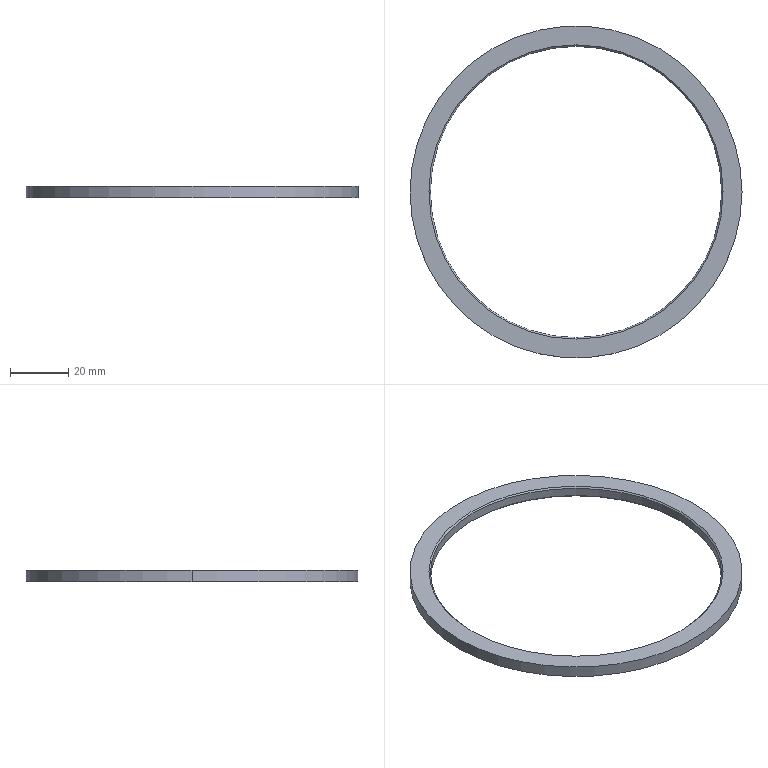Part | SolidWorks | features Revolution 1 | 1 solid | 10 faces | box 114 x 114 x 4 mm | volume 9333 mm3 | cone 4 | cylinder 4 | plane 2 | commonest cylinder face diameters 100 x2 114 x2
STEP:
#1=CARTESIAN_POINT('',(471.231,234.744,-188.193));
#2=VERTEX_POINT('',#1);
#3=CARTESIAN_POINT('',(571.231,234.744,-188.193));
#4=VERTEX_POINT('',#3);
#5=CARTESIAN_POINT('',(521.231,234.744,-188.193));
#6=DIRECTION('',(0.,0.,1.));
#7=DIRECTION('',(1.,0.,0.));
#8=AXIS2_PLACEMENT_3D('',#5,#6,#7);
#9=CIRCLE('',#8,50.);
#10=EDGE_CURVE('',#2,#4,#9,.T.);
#11=ORIENTED_EDGE('',*,*,#10,.T.);
#12=CARTESIAN_POINT('',(571.731,234.744,-188.693));
#13=VERTEX_POINT('',#12);
#14=CARTESIAN_POINT('',(571.731,234.744,-188.693));
#15=DIRECTION('',(0.7071,0.,-0.7071));
#16=VECTOR('',#15,1000.);
#17=LINE('',#14,#16);
#18=EDGE_CURVE('',#4,#13,#17,.T.);
#19=ORIENTED_EDGE('',*,*,#18,.T.);
#20=CARTESIAN_POINT('',(470.731,234.744,-188.693));
#21=VERTEX_POINT('',#20);
#22=CARTESIAN_POINT('',(521.231,234.744,-188.693));
#23=DIRECTION('',(0.,0.,1.));
#24=DIRECTION('',(1.,0.,0.));
#25=AXIS2_PLACEMENT_3D('',#22,#23,#24);
#26=CIRCLE('',#25,50.5);
#27=EDGE_CURVE('',#21,#13,#26,.T.);
#28=ORIENTED_EDGE('',*,*,#27,.F.);
#29=CARTESIAN_POINT('',(470.731,234.744,-188.693));
#30=DIRECTION('',(-0.7071,0.,-0.7071));
#31=VECTOR('',#30,1000.);
#32=LINE('',#29,#31);
#33=EDGE_CURVE('',#2,#21,#32,.T.);
#34=ORIENTED_EDGE('',*,*,#33,.F.);
#35=EDGE_LOOP('',(#11,#19,#28,#34));
#36=FACE_OUTER_BOUND('',#35,.T.);
#37=CARTESIAN_POINT('',(521.231,234.744,-188.693));
#38=DIRECTION('',(0.,0.,-1.));
#39=DIRECTION('',(-1.,0.,0.));
#40=AXIS2_PLACEMENT_3D('',#37,#38,#39);
#41=CONICAL_SURFACE('',#40,50.5,0.7854);
#42=ADVANCED_FACE('',(#36),#41,.F.);
#43=CARTESIAN_POINT('',(578.231,234.744,-188.693));
#44=VERTEX_POINT('',#43);
#45=CARTESIAN_POINT('',(464.231,234.744,-188.693));
#46=VERTEX_POINT('',#45);
#47=CARTESIAN_POINT('',(521.231,234.744,-188.693));
#48=DIRECTION('',(0.,0.,1.));
#49=DIRECTION('',(1.,0.,0.));
#50=AXIS2_PLACEMENT_3D('',#47,#48,#49);
#51=CIRCLE('',#50,57.);
#52=EDGE_CURVE('',#44,#46,#51,.T.);
#53=ORIENTED_EDGE('',*,*,#52,.T.);
#54=CARTESIAN_POINT('',(464.231,234.744,-184.693));
#55=VERTEX_POINT('',#54);
#56=CARTESIAN_POINT('',(464.231,234.744,-188.693));
#57=DIRECTION('',(0.,0.,1.));
#58=VECTOR('',#57,1000.);
#59=LINE('',#56,#58);
#60=EDGE_CURVE('',#46,#55,#59,.T.);
#61=ORIENTED_EDGE('',*,*,#60,.T.);
#62=CARTESIAN_POINT('',(578.231,234.744,-184.693));
#63=VERTEX_POINT('',#62);
#64=CARTESIAN_POINT('',(521.231,234.744,-184.693));
#65=DIRECTION('',(0.,0.,1.));
#66=DIRECTION('',(1.,0.,0.));
#67=AXIS2_PLACEMENT_3D('',#64,#65,#66);
#68=CIRCLE('',#67,57.);
#69=EDGE_CURVE('',#63,#55,#68,.T.);
#70=ORIENTED_EDGE('',*,*,#69,.F.);
#71=CARTESIAN_POINT('',(578.231,234.744,-188.693));
#72=DIRECTION('',(0.,0.,1.));
#73=VECTOR('',#72,1000.);
#74=LINE('',#71,#73);
#75=EDGE_CURVE('',#44,#63,#74,.T.);
#76=ORIENTED_EDGE('',*,*,#75,.F.);
#77=EDGE_LOOP('',(#53,#61,#70,#76));
#78=FACE_OUTER_BOUND('',#77,.T.);
#79=CARTESIAN_POINT('',(521.231,234.744,-188.693));
#80=DIRECTION('',(0.,0.,1.));
#81=DIRECTION('',(1.,0.,0.));
#82=AXIS2_PLACEMENT_3D('',#79,#80,#81);
#83=CYLINDRICAL_SURFACE('',#82,57.);
#84=ADVANCED_FACE('',(#78),#83,.T.);
#85=CARTESIAN_POINT('',(471.231,234.744,-185.193));
#86=VERTEX_POINT('',#85);
#87=CARTESIAN_POINT('',(571.231,234.744,-185.193));
#88=VERTEX_POINT('',#87);
#89=CARTESIAN_POINT('',(521.231,234.744,-185.193));
#90=DIRECTION('',(0.,0.,1.));
#91=DIRECTION('',(1.,0.,0.));
#92=AXIS2_PLACEMENT_3D('',#89,#90,#91);
#93=CIRCLE('',#92,50.);
#94=EDGE_CURVE('',#86,#88,#93,.T.);
#95=ORIENTED_EDGE('',*,*,#94,.F.);
#96=CARTESIAN_POINT('',(470.731,234.744,-184.693));
#97=VERTEX_POINT('',#96);
#98=CARTESIAN_POINT('',(471.231,234.744,-185.193));
#99=DIRECTION('',(-0.7071,0.,0.7071));
#100=VECTOR('',#99,1000.);
#101=LINE('',#98,#100);
#102=EDGE_CURVE('',#86,#97,#101,.T.);
#103=ORIENTED_EDGE('',*,*,#102,.T.);
#104=CARTESIAN_POINT('',(571.731,234.744,-184.693));
#105=VERTEX_POINT('',#104);
#106=CARTESIAN_POINT('',(521.231,234.744,-184.693));
#107=DIRECTION('',(0.,0.,1.));
#108=DIRECTION('',(1.,0.,0.));
#109=AXIS2_PLACEMENT_3D('',#106,#107,#108);
#110=CIRCLE('',#109,50.5);
#111=EDGE_CURVE('',#97,#105,#110,.T.);
#112=ORIENTED_EDGE('',*,*,#111,.T.);
#113=CARTESIAN_POINT('',(571.231,234.744,-185.193));
#114=DIRECTION('',(0.7071,0.,0.7071));
#115=VECTOR('',#114,1000.);
#116=LINE('',#113,#115);
#117=EDGE_CURVE('',#88,#105,#116,.T.);
#118=ORIENTED_EDGE('',*,*,#117,.F.);
#119=EDGE_LOOP('',(#95,#103,#112,#118));
#120=FACE_OUTER_BOUND('',#119,.T.);
#121=CARTESIAN_POINT('',(521.231,234.744,-185.193));
#122=DIRECTION('',(0.,0.,1.));
#123=DIRECTION('',(1.,0.,0.));
#124=AXIS2_PLACEMENT_3D('',#121,#122,#123);
#125=CONICAL_SURFACE('',#124,50.,0.7854);
#126=ADVANCED_FACE('',(#120),#125,.F.);
#127=ORIENTED_EDGE('',*,*,#10,.F.);
#128=CARTESIAN_POINT('',(471.231,234.744,-188.693));
#129=DIRECTION('',(0.,0.,1.));
#130=VECTOR('',#129,1000.);
#131=LINE('',#128,#130);
#132=EDGE_CURVE('',#2,#86,#131,.T.);
#133=ORIENTED_EDGE('',*,*,#132,.T.);
#134=ORIENTED_EDGE('',*,*,#94,.T.);
#135=CARTESIAN_POINT('',(571.231,234.744,-188.693));
#136=DIRECTION('',(0.,0.,1.));
#137=VECTOR('',#136,1000.);
#138=LINE('',#135,#137);
#139=EDGE_CURVE('',#4,#88,#138,.T.);
#140=ORIENTED_EDGE('',*,*,#139,.F.);
#141=EDGE_LOOP('',(#127,#133,#134,#140));
#142=FACE_OUTER_BOUND('',#141,.T.);
#143=CARTESIAN_POINT('',(521.231,234.744,-188.693));
#144=DIRECTION('',(0.,0.,1.));
#145=DIRECTION('',(1.,0.,0.));
#146=AXIS2_PLACEMENT_3D('',#143,#144,#145);
#147=CYLINDRICAL_SURFACE('',#146,50.);
#148=ADVANCED_FACE('',(#142),#147,.F.);
#149=ORIENTED_EDGE('',*,*,#132,.F.);
#150=CARTESIAN_POINT('',(521.231,234.744,-188.193));
#151=DIRECTION('',(0.,0.,1.));
#152=DIRECTION('',(1.,0.,0.));
#153=AXIS2_PLACEMENT_3D('',#150,#151,#152);
#154=CIRCLE('',#153,50.);
#155=EDGE_CURVE('',#4,#2,#154,.T.);
#156=ORIENTED_EDGE('',*,*,#155,.F.);
#157=ORIENTED_EDGE('',*,*,#139,.T.);
#158=CARTESIAN_POINT('',(521.231,234.744,-185.193));
#159=DIRECTION('',(0.,0.,1.));
#160=DIRECTION('',(1.,0.,0.));
#161=AXIS2_PLACEMENT_3D('',#158,#159,#160);
#162=CIRCLE('',#161,50.);
#163=EDGE_CURVE('',#88,#86,#162,.T.);
#164=ORIENTED_EDGE('',*,*,#163,.T.);
#165=EDGE_LOOP('',(#149,#156,#157,#164));
#166=FACE_OUTER_BOUND('',#165,.T.);
#167=CARTESIAN_POINT('',(521.231,234.744,-188.693));
#168=DIRECTION('',(0.,0.,1.));
#169=DIRECTION('',(1.,0.,0.));
#170=AXIS2_PLACEMENT_3D('',#167,#168,#169);
#171=CYLINDRICAL_SURFACE('',#170,50.);
#172=ADVANCED_FACE('',(#166),#171,.F.);
#173=ORIENTED_EDGE('',*,*,#102,.F.);
#174=ORIENTED_EDGE('',*,*,#163,.F.);
#175=ORIENTED_EDGE('',*,*,#117,.T.);
#176=CARTESIAN_POINT('',(521.231,234.744,-184.693));
#177=DIRECTION('',(0.,0.,1.));
#178=DIRECTION('',(1.,0.,0.));
#179=AXIS2_PLACEMENT_3D('',#176,#177,#178);
#180=CIRCLE('',#179,50.5);
#181=EDGE_CURVE('',#105,#97,#180,.T.);
#182=ORIENTED_EDGE('',*,*,#181,.T.);
#183=EDGE_LOOP('',(#173,#174,#175,#182));
#184=FACE_OUTER_BOUND('',#183,.T.);
#185=CARTESIAN_POINT('',(521.231,234.744,-185.193));
#186=DIRECTION('',(0.,0.,1.));
#187=DIRECTION('',(1.,0.,0.));
#188=AXIS2_PLACEMENT_3D('',#185,#186,#187);
#189=CONICAL_SURFACE('',#188,50.,0.7854);
#190=ADVANCED_FACE('',(#184),#189,.F.);
#191=ORIENTED_EDGE('',*,*,#69,.T.);
#192=CARTESIAN_POINT('',(521.231,234.744,-184.693));
#193=DIRECTION('',(0.,0.,1.));
#194=DIRECTION('',(1.,0.,0.));
#195=AXIS2_PLACEMENT_3D('',#192,#193,#194);
#196=CIRCLE('',#195,57.);
#197=EDGE_CURVE('',#55,#63,#196,.T.);
#198=ORIENTED_EDGE('',*,*,#197,.T.);
#199=EDGE_LOOP('',(#191,#198));
#200=FACE_OUTER_BOUND('',#199,.T.);
#201=ORIENTED_EDGE('',*,*,#181,.F.);
#202=ORIENTED_EDGE('',*,*,#111,.F.);
#203=EDGE_LOOP('',(#201,#202));
#204=FACE_BOUND('',#203,.T.);
#205=CARTESIAN_POINT('',(571.731,234.744,-184.693));
#206=DIRECTION('',(0.,0.,1.));
#207=DIRECTION('',(1.,0.,0.));
#208=AXIS2_PLACEMENT_3D('',#205,#206,#207);
#209=PLANE('',#208);
#210=ADVANCED_FACE('',(#200,#204),#209,.T.);
#211=ORIENTED_EDGE('',*,*,#60,.F.);
#212=CARTESIAN_POINT('',(521.231,234.744,-188.693));
#213=DIRECTION('',(0.,0.,1.));
#214=DIRECTION('',(1.,0.,0.));
#215=AXIS2_PLACEMENT_3D('',#212,#213,#214);
#216=CIRCLE('',#215,57.);
#217=EDGE_CURVE('',#46,#44,#216,.T.);
#218=ORIENTED_EDGE('',*,*,#217,.T.);
#219=ORIENTED_EDGE('',*,*,#75,.T.);
#220=ORIENTED_EDGE('',*,*,#197,.F.);
#221=EDGE_LOOP('',(#211,#218,#219,#220));
#222=FACE_OUTER_BOUND('',#221,.T.);
#223=CARTESIAN_POINT('',(521.231,234.744,-188.693));
#224=DIRECTION('',(0.,0.,1.));
#225=DIRECTION('',(1.,0.,0.));
#226=AXIS2_PLACEMENT_3D('',#223,#224,#225);
#227=CYLINDRICAL_SURFACE('',#226,57.);
#228=ADVANCED_FACE('',(#222),#227,.T.);
#229=ORIENTED_EDGE('',*,*,#27,.T.);
#230=CARTESIAN_POINT('',(521.231,234.744,-188.693));
#231=DIRECTION('',(0.,0.,1.));
#232=DIRECTION('',(1.,0.,0.));
#233=AXIS2_PLACEMENT_3D('',#230,#231,#232);
#234=CIRCLE('',#233,50.5);
#235=EDGE_CURVE('',#13,#21,#234,.T.);
#236=ORIENTED_EDGE('',*,*,#235,.T.);
#237=EDGE_LOOP('',(#229,#236));
#238=FACE_BOUND('',#237,.T.);
#239=ORIENTED_EDGE('',*,*,#52,.F.);
#240=ORIENTED_EDGE('',*,*,#217,.F.);
#241=EDGE_LOOP('',(#239,#240));
#242=FACE_OUTER_BOUND('',#241,.T.);
#243=CARTESIAN_POINT('',(578.231,234.744,-188.693));
#244=DIRECTION('',(0.,0.,-1.));
#245=DIRECTION('',(-1.,0.,0.));
#246=AXIS2_PLACEMENT_3D('',#243,#244,#245);
#247=PLANE('',#246);
#248=ADVANCED_FACE('',(#238,#242),#247,.T.);
#249=ORIENTED_EDGE('',*,*,#18,.F.);
#250=ORIENTED_EDGE('',*,*,#155,.T.);
#251=ORIENTED_EDGE('',*,*,#33,.T.);
#252=ORIENTED_EDGE('',*,*,#235,.F.);
#253=EDGE_LOOP('',(#249,#250,#251,#252));
#254=FACE_OUTER_BOUND('',#253,.T.);
#255=CARTESIAN_POINT('',(521.231,234.744,-188.693));
#256=DIRECTION('',(0.,0.,-1.));
#257=DIRECTION('',(-1.,0.,0.));
#258=AXIS2_PLACEMENT_3D('',#255,#256,#257);
#259=CONICAL_SURFACE('',#258,50.5,0.7854);
#260=ADVANCED_FACE('',(#254),#259,.F.);
#261=CLOSED_SHELL('',(#42,#84,#126,#148,#172,#190,#210,#228,#248,#260));
#262=MANIFOLD_SOLID_BREP('',#261);
#263=CARTESIAN_POINT('',(0.,0.,0.));
#264=DIRECTION('',(0.,0.,1.));
#265=DIRECTION('',(1.,0.,0.));
#266=AXIS2_PLACEMENT_3D('',#263,#264,#265);
#267=(LENGTH_UNIT()NAMED_UNIT(*)SI_UNIT(.MILLI.,.METRE.));
#268=UNCERTAINTY_MEASURE_WITH_UNIT(LENGTH_MEASURE(0.00001),#267,'','');
#269=(NAMED_UNIT(*)PLANE_ANGLE_UNIT()SI_UNIT($,.RADIAN.));
#270=(NAMED_UNIT(*)SI_UNIT($,.STERADIAN.)SOLID_ANGLE_UNIT());
#271=(GEOMETRIC_REPRESENTATION_CONTEXT(3)GLOBAL_UNCERTAINTY_ASSIGNED_CONTEXT((#268))GLOBAL_UNIT_ASSIGNED_CONTEXT((#267,#269,#270))REPRESENTATION_CONTEXT('',''));
#272=ADVANCED_BREP_SHAPE_REPRESENTATION('',(#262,#266),#271);